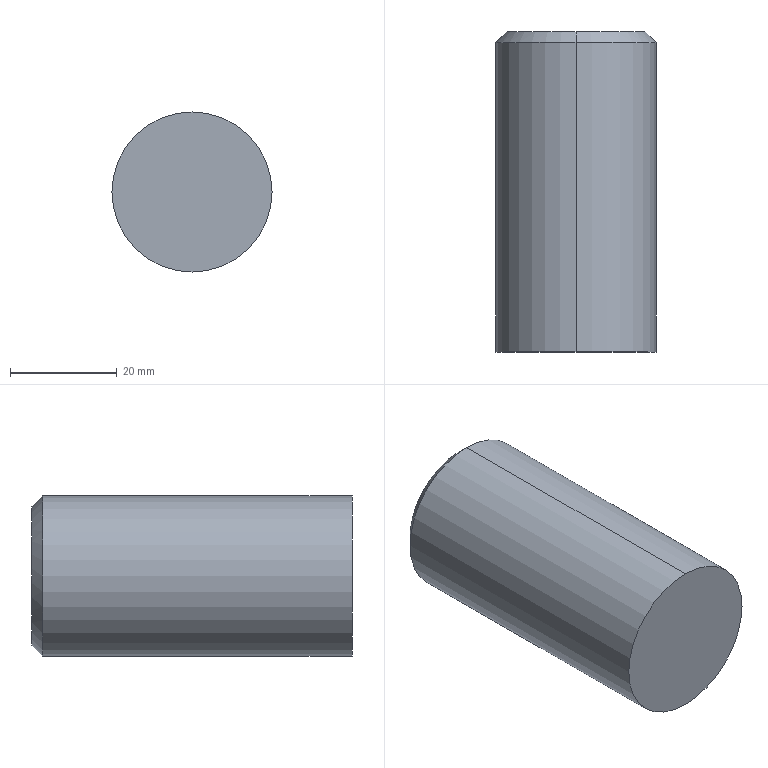Part | SolidWorks | features BaseBody 1 | 1 solid | 6 faces | box 30 x 60 x 30 mm | volume 42231 mm3 | cylinder 2 | cone 2 | plane 2 | commonest cylinder face diameters 30 x2
STEP:
#1=CARTESIAN_POINT('',(57.247,354.5,-51.));
#2=VERTEX_POINT('',#1);
#3=CARTESIAN_POINT('',(57.247,354.5,-81.));
#4=VERTEX_POINT('',#3);
#5=CARTESIAN_POINT('',(57.247,354.5,-66.));
#6=DIRECTION('',(0.,1.,0.));
#7=DIRECTION('',(0.,0.,1.));
#8=AXIS2_PLACEMENT_3D('',#5,#6,#7);
#9=CIRCLE('',#8,15.);
#10=EDGE_CURVE('',#2,#4,#9,.T.);
#11=ORIENTED_EDGE('',*,*,#10,.T.);
#12=CARTESIAN_POINT('',(57.247,412.5,-81.));
#13=VERTEX_POINT('',#12);
#14=CARTESIAN_POINT('',(57.247,389.5,-81.));
#15=DIRECTION('',(0.,1.,0.));
#16=VECTOR('',#15,1000.);
#17=LINE('',#14,#16);
#18=EDGE_CURVE('',#4,#13,#17,.T.);
#19=ORIENTED_EDGE('',*,*,#18,.T.);
#20=CARTESIAN_POINT('',(57.247,412.5,-51.));
#21=VERTEX_POINT('',#20);
#22=CARTESIAN_POINT('',(57.247,412.5,-66.));
#23=DIRECTION('',(0.,-1.,0.));
#24=DIRECTION('',(0.,0.,1.));
#25=AXIS2_PLACEMENT_3D('',#22,#23,#24);
#26=CIRCLE('',#25,15.);
#27=EDGE_CURVE('',#13,#21,#26,.T.);
#28=ORIENTED_EDGE('',*,*,#27,.T.);
#29=CARTESIAN_POINT('',(57.247,389.5,-51.));
#30=DIRECTION('',(0.,1.,0.));
#31=VECTOR('',#30,1000.);
#32=LINE('',#29,#31);
#33=EDGE_CURVE('',#2,#21,#32,.T.);
#34=ORIENTED_EDGE('',*,*,#33,.F.);
#35=EDGE_LOOP('',(#11,#19,#28,#34));
#36=FACE_OUTER_BOUND('',#35,.T.);
#37=CARTESIAN_POINT('',(57.247,389.5,-66.));
#38=DIRECTION('',(0.,1.,0.));
#39=DIRECTION('',(0.,0.,1.));
#40=AXIS2_PLACEMENT_3D('',#37,#38,#39);
#41=CYLINDRICAL_SURFACE('',#40,15.);
#42=ADVANCED_FACE('',(#36),#41,.T.);
#43=CARTESIAN_POINT('',(57.247,414.5,-79.));
#44=VERTEX_POINT('',#43);
#45=CARTESIAN_POINT('',(57.247,414.5,-53.));
#46=VERTEX_POINT('',#45);
#47=CARTESIAN_POINT('',(57.247,414.5,-66.));
#48=DIRECTION('',(0.,-1.,0.));
#49=DIRECTION('',(0.,0.,-1.));
#50=AXIS2_PLACEMENT_3D('',#47,#48,#49);
#51=CIRCLE('',#50,13.);
#52=EDGE_CURVE('',#44,#46,#51,.T.);
#53=ORIENTED_EDGE('',*,*,#52,.T.);
#54=CARTESIAN_POINT('',(57.247,412.5,-51.));
#55=DIRECTION('',(0.,-0.7071,0.7071));
#56=VECTOR('',#55,1000.);
#57=LINE('',#54,#56);
#58=EDGE_CURVE('',#46,#21,#57,.T.);
#59=ORIENTED_EDGE('',*,*,#58,.T.);
#60=ORIENTED_EDGE('',*,*,#27,.F.);
#61=CARTESIAN_POINT('',(57.247,412.5,-81.));
#62=DIRECTION('',(0.,-0.7071,-0.7071));
#63=VECTOR('',#62,1000.);
#64=LINE('',#61,#63);
#65=EDGE_CURVE('',#44,#13,#64,.T.);
#66=ORIENTED_EDGE('',*,*,#65,.F.);
#67=EDGE_LOOP('',(#53,#59,#60,#66));
#68=FACE_OUTER_BOUND('',#67,.T.);
#69=CARTESIAN_POINT('',(57.247,412.5,-66.));
#70=DIRECTION('',(0.,-1.,0.));
#71=DIRECTION('',(0.,0.,-1.));
#72=AXIS2_PLACEMENT_3D('',#69,#70,#71);
#73=CONICAL_SURFACE('',#72,15.,0.7854);
#74=ADVANCED_FACE('',(#68),#73,.T.);
#75=ORIENTED_EDGE('',*,*,#18,.F.);
#76=CARTESIAN_POINT('',(57.247,354.5,-66.));
#77=DIRECTION('',(0.,1.,0.));
#78=DIRECTION('',(0.,0.,1.));
#79=AXIS2_PLACEMENT_3D('',#76,#77,#78);
#80=CIRCLE('',#79,15.);
#81=EDGE_CURVE('',#4,#2,#80,.T.);
#82=ORIENTED_EDGE('',*,*,#81,.T.);
#83=ORIENTED_EDGE('',*,*,#33,.T.);
#84=CARTESIAN_POINT('',(57.247,412.5,-66.));
#85=DIRECTION('',(0.,-1.,0.));
#86=DIRECTION('',(0.,0.,1.));
#87=AXIS2_PLACEMENT_3D('',#84,#85,#86);
#88=CIRCLE('',#87,15.);
#89=EDGE_CURVE('',#21,#13,#88,.T.);
#90=ORIENTED_EDGE('',*,*,#89,.T.);
#91=EDGE_LOOP('',(#75,#82,#83,#90));
#92=FACE_OUTER_BOUND('',#91,.T.);
#93=CARTESIAN_POINT('',(57.247,389.5,-66.));
#94=DIRECTION('',(0.,1.,0.));
#95=DIRECTION('',(0.,0.,1.));
#96=AXIS2_PLACEMENT_3D('',#93,#94,#95);
#97=CYLINDRICAL_SURFACE('',#96,15.);
#98=ADVANCED_FACE('',(#92),#97,.T.);
#99=ORIENTED_EDGE('',*,*,#58,.F.);
#100=CARTESIAN_POINT('',(57.247,414.5,-66.));
#101=DIRECTION('',(0.,-1.,0.));
#102=DIRECTION('',(0.,0.,-1.));
#103=AXIS2_PLACEMENT_3D('',#100,#101,#102);
#104=CIRCLE('',#103,13.);
#105=EDGE_CURVE('',#46,#44,#104,.T.);
#106=ORIENTED_EDGE('',*,*,#105,.T.);
#107=ORIENTED_EDGE('',*,*,#65,.T.);
#108=ORIENTED_EDGE('',*,*,#89,.F.);
#109=EDGE_LOOP('',(#99,#106,#107,#108));
#110=FACE_OUTER_BOUND('',#109,.T.);
#111=CARTESIAN_POINT('',(57.247,412.5,-66.));
#112=DIRECTION('',(0.,-1.,0.));
#113=DIRECTION('',(0.,0.,-1.));
#114=AXIS2_PLACEMENT_3D('',#111,#112,#113);
#115=CONICAL_SURFACE('',#114,15.,0.7854);
#116=ADVANCED_FACE('',(#110),#115,.T.);
#117=ORIENTED_EDGE('',*,*,#10,.F.);
#118=ORIENTED_EDGE('',*,*,#81,.F.);
#119=EDGE_LOOP('',(#117,#118));
#120=FACE_OUTER_BOUND('',#119,.T.);
#121=CARTESIAN_POINT('',(31.631,354.5,-284.615));
#122=DIRECTION('',(0.,-1.,0.));
#123=DIRECTION('',(0.,0.,-1.));
#124=AXIS2_PLACEMENT_3D('',#121,#122,#123);
#125=PLANE('',#124);
#126=ADVANCED_FACE('',(#120),#125,.T.);
#127=ORIENTED_EDGE('',*,*,#52,.F.);
#128=ORIENTED_EDGE('',*,*,#105,.F.);
#129=EDGE_LOOP('',(#127,#128));
#130=FACE_OUTER_BOUND('',#129,.T.);
#131=CARTESIAN_POINT('',(57.247,414.5,-66.));
#132=DIRECTION('',(0.,1.,0.));
#133=DIRECTION('',(0.,0.,1.));
#134=AXIS2_PLACEMENT_3D('',#131,#132,#133);
#135=PLANE('',#134);
#136=ADVANCED_FACE('',(#130),#135,.T.);
#137=CLOSED_SHELL('',(#42,#74,#98,#116,#126,#136));
#138=MANIFOLD_SOLID_BREP('',#137);
#139=CARTESIAN_POINT('',(0.,0.,0.));
#140=DIRECTION('',(0.,0.,1.));
#141=DIRECTION('',(1.,0.,0.));
#142=AXIS2_PLACEMENT_3D('',#139,#140,#141);
#143=(LENGTH_UNIT()NAMED_UNIT(*)SI_UNIT(.MILLI.,.METRE.));
#144=UNCERTAINTY_MEASURE_WITH_UNIT(LENGTH_MEASURE(0.00001),#143,'','');
#145=(NAMED_UNIT(*)PLANE_ANGLE_UNIT()SI_UNIT($,.RADIAN.));
#146=(NAMED_UNIT(*)SI_UNIT($,.STERADIAN.)SOLID_ANGLE_UNIT());
#147=(GEOMETRIC_REPRESENTATION_CONTEXT(3)GLOBAL_UNCERTAINTY_ASSIGNED_CONTEXT((#144))GLOBAL_UNIT_ASSIGNED_CONTEXT((#143,#145,#146))REPRESENTATION_CONTEXT('',''));
#148=ADVANCED_BREP_SHAPE_REPRESENTATION('',(#138,#142),#147);